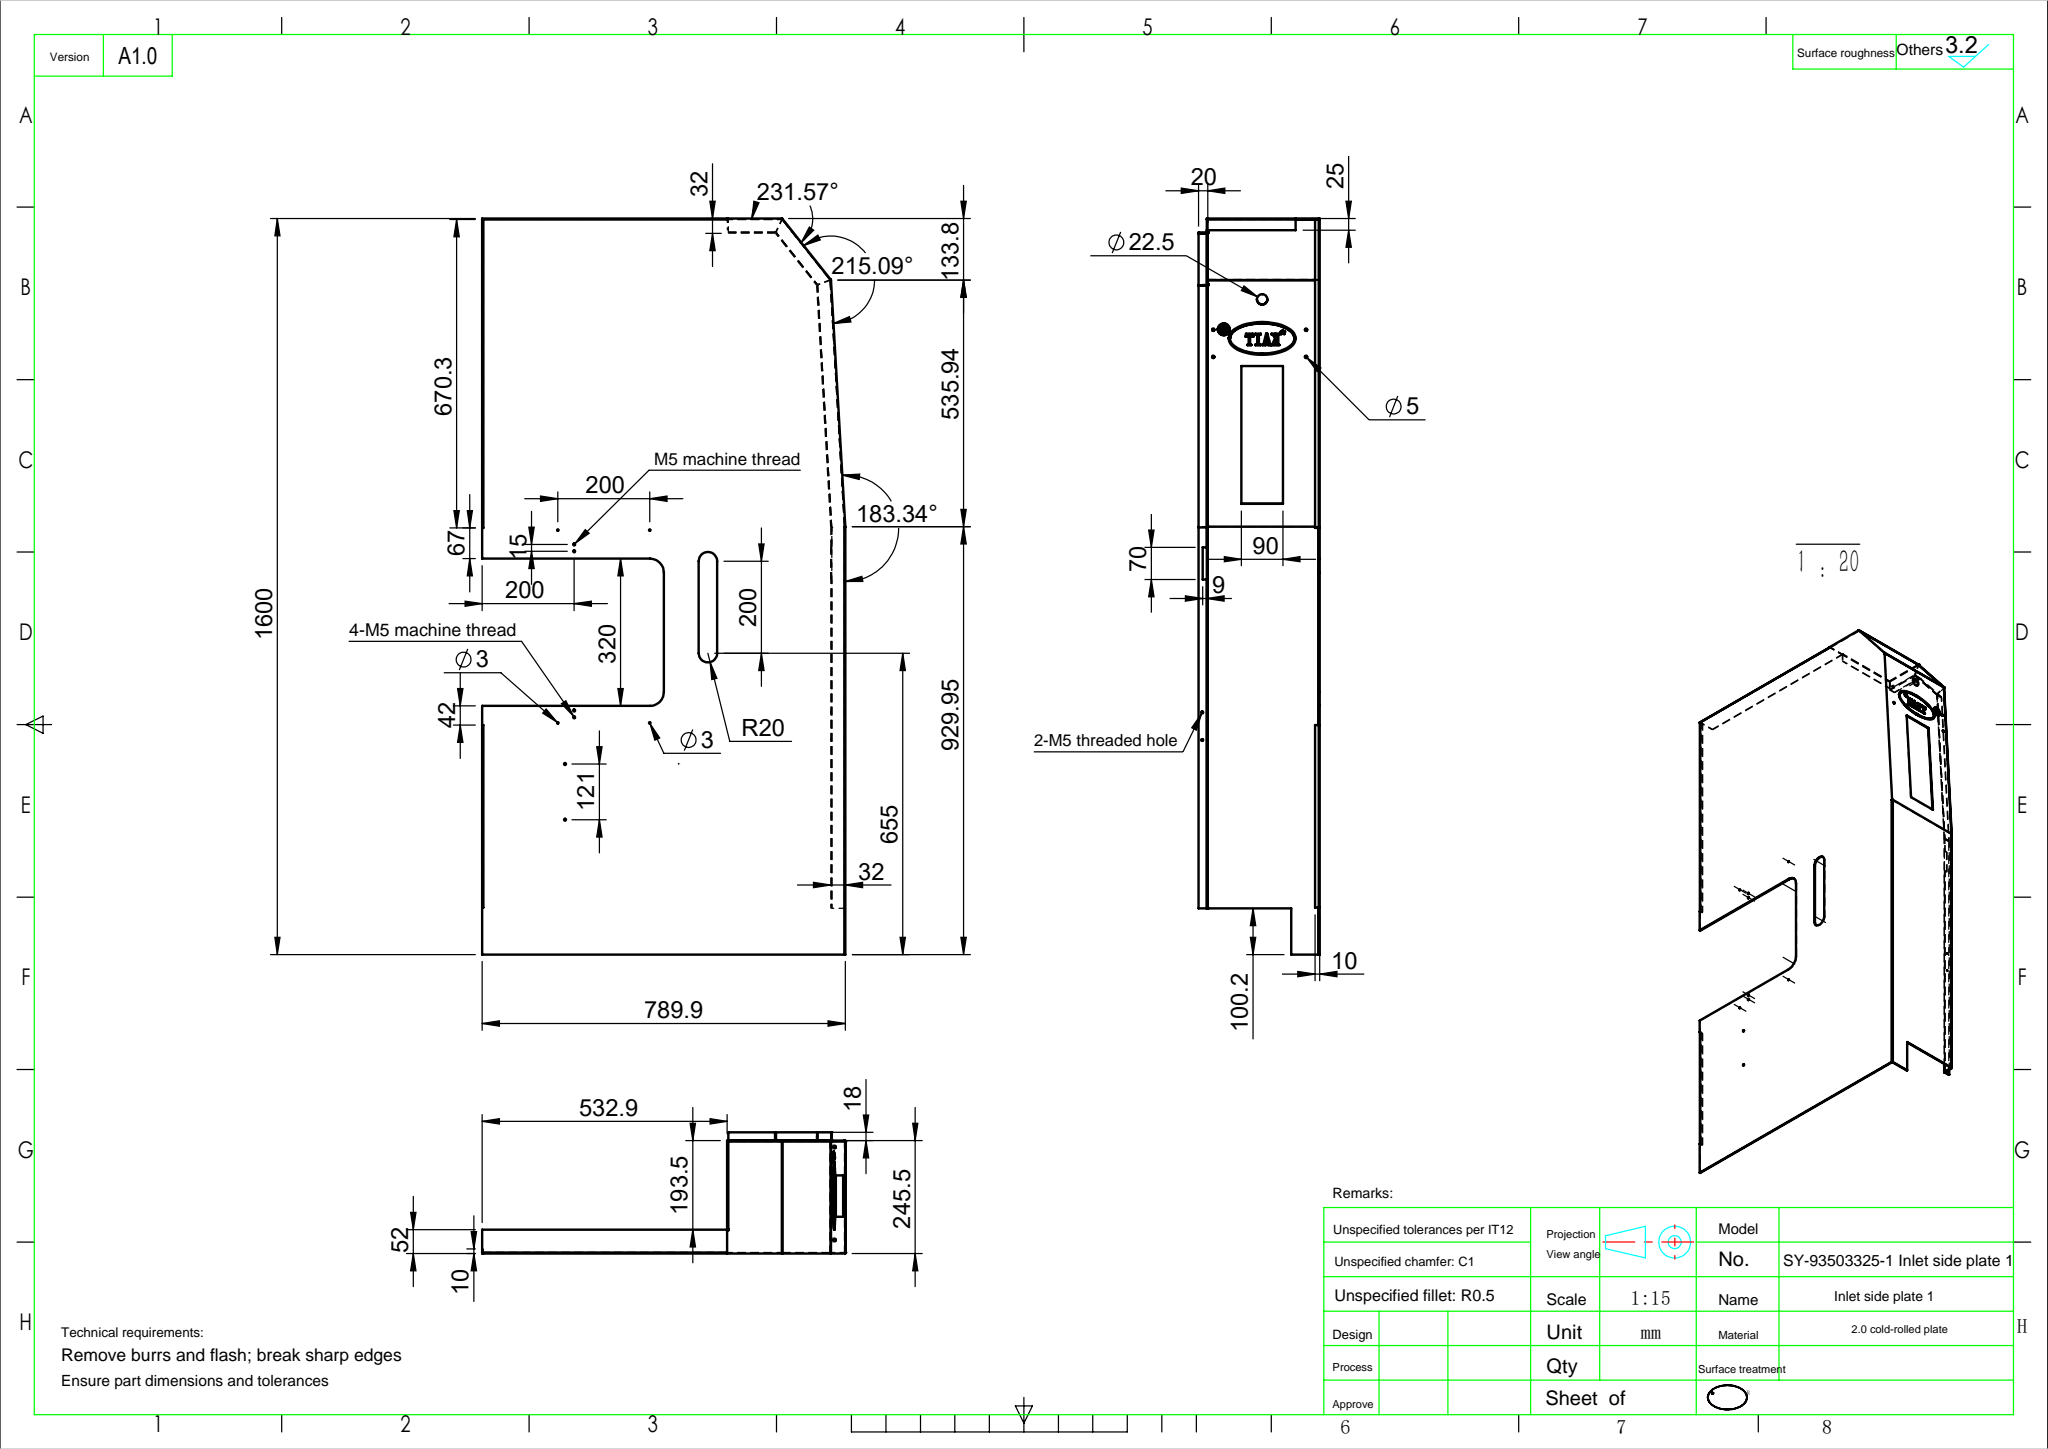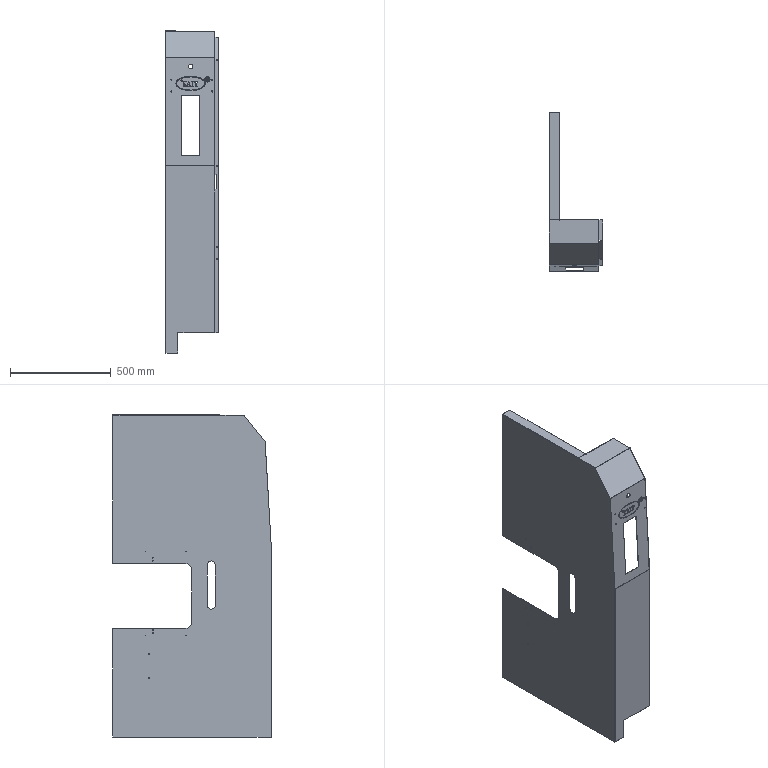Part | SolidWorks | features ICE 19, EdgeFlange 8, Cut 5, 3DProfileFeature 3, HoleWzd 3, FlatPattern 2, SMBaseFlange 2, SheetMetal 2 | 2 solids | 389 faces | box 263.5 x 789.9 x 1600 mm | volume 3203804 mm3 | plane 257 | cylinder 86 | spline 42 | cone 4 | commonest cylinder face diameters 0.4 x16 4.2 x16 4.4 x15 1 x8 3 x8 5 x8